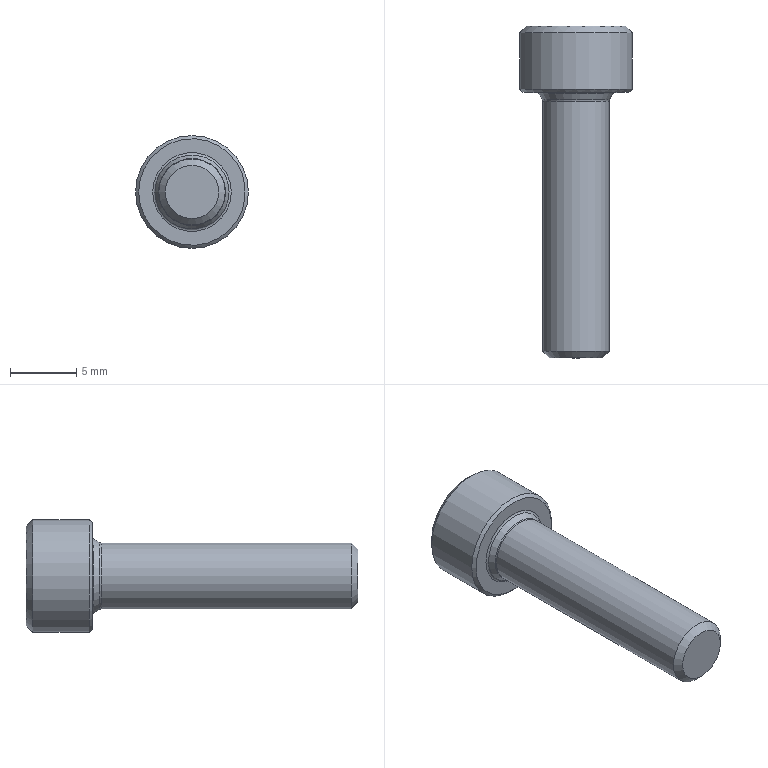Part | STEP file | 1 solid | 31 faces | box 8.5 x 25 x 8.5 mm | volume 625.305 mm3 | plane 15 | cone 11 | cylinder 3 | torus 2 | commonest cylinder face diameters 4 x1 5 x1 8.5 x1